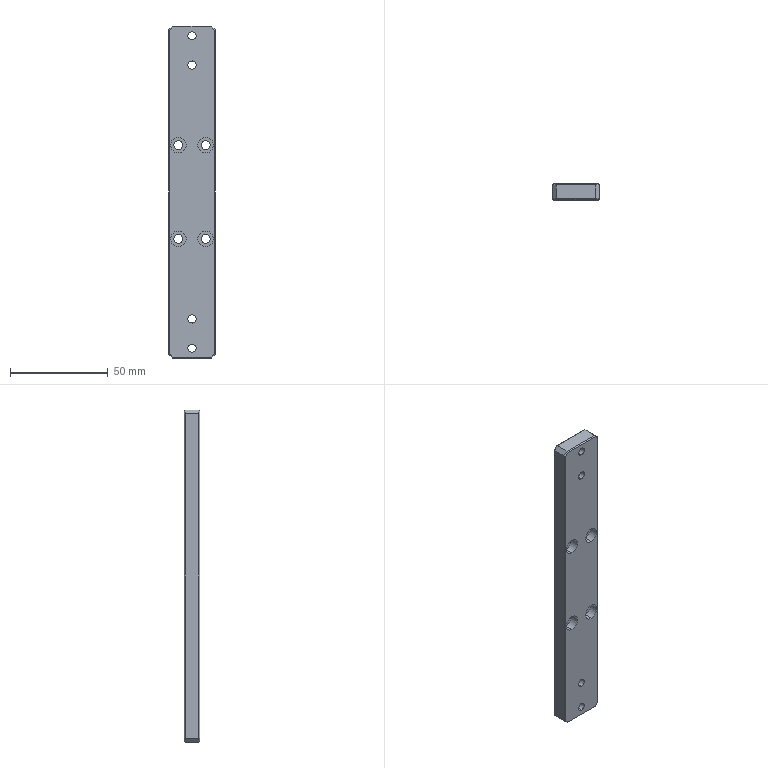Part | SolidWorks | features Chamfer 2, HoleWzd 2, Extrusion 1 | 1 solid | 54 faces | box 24 x 8 x 170 mm | volume 30923 mm3 | plane 30 | cylinder 24 | commonest cylinder face diameters 4.2 x8 4.5 x8 8 x8
STEP:
#1=CARTESIAN_POINT('',(0.,0.,-82.1));
#2=VERTEX_POINT('',#1);
#3=CARTESIAN_POINT('',(0.,0.,-77.9));
#4=VERTEX_POINT('',#3);
#5=CARTESIAN_POINT('',(0.,0.,-80.));
#6=DIRECTION('',(0.,1.,0.));
#7=DIRECTION('',(0.,0.,1.));
#8=AXIS2_PLACEMENT_3D('',#5,#6,#7);
#9=CIRCLE('',#8,2.1);
#10=EDGE_CURVE('',#2,#4,#9,.T.);
#11=ORIENTED_EDGE('',*,*,#10,.F.);
#12=CARTESIAN_POINT('',(0.,8.,-82.1));
#13=VERTEX_POINT('',#12);
#14=CARTESIAN_POINT('',(0.,8.,-82.1));
#15=DIRECTION('',(0.,1.,0.));
#16=VECTOR('',#15,1000.);
#17=LINE('',#14,#16);
#18=EDGE_CURVE('',#2,#13,#17,.T.);
#19=ORIENTED_EDGE('',*,*,#18,.T.);
#20=CARTESIAN_POINT('',(0.,8.,-77.9));
#21=VERTEX_POINT('',#20);
#22=CARTESIAN_POINT('',(0.,8.,-80.));
#23=DIRECTION('',(0.,1.,0.));
#24=DIRECTION('',(0.,0.,1.));
#25=AXIS2_PLACEMENT_3D('',#22,#23,#24);
#26=CIRCLE('',#25,2.1);
#27=EDGE_CURVE('',#13,#21,#26,.T.);
#28=ORIENTED_EDGE('',*,*,#27,.T.);
#29=CARTESIAN_POINT('',(0.,8.,-77.9));
#30=DIRECTION('',(0.,1.,0.));
#31=VECTOR('',#30,1000.);
#32=LINE('',#29,#31);
#33=EDGE_CURVE('',#4,#21,#32,.T.);
#34=ORIENTED_EDGE('',*,*,#33,.F.);
#35=EDGE_LOOP('',(#11,#19,#28,#34));
#36=FACE_OUTER_BOUND('',#35,.T.);
#37=CARTESIAN_POINT('',(0.,8.,-80.));
#38=DIRECTION('',(0.,1.,0.));
#39=DIRECTION('',(0.,0.,1.));
#40=AXIS2_PLACEMENT_3D('',#37,#38,#39);
#41=CYLINDRICAL_SURFACE('',#40,2.1);
#42=ADVANCED_FACE('',(#36),#41,.F.);
#43=CARTESIAN_POINT('',(0.,0.,77.9));
#44=VERTEX_POINT('',#43);
#45=CARTESIAN_POINT('',(0.,0.,82.1));
#46=VERTEX_POINT('',#45);
#47=CARTESIAN_POINT('',(0.,0.,80.));
#48=DIRECTION('',(0.,1.,0.));
#49=DIRECTION('',(0.,0.,1.));
#50=AXIS2_PLACEMENT_3D('',#47,#48,#49);
#51=CIRCLE('',#50,2.1);
#52=EDGE_CURVE('',#44,#46,#51,.T.);
#53=ORIENTED_EDGE('',*,*,#52,.F.);
#54=CARTESIAN_POINT('',(0.,8.,77.9));
#55=VERTEX_POINT('',#54);
#56=CARTESIAN_POINT('',(0.,8.,77.9));
#57=DIRECTION('',(0.,1.,0.));
#58=VECTOR('',#57,1000.);
#59=LINE('',#56,#58);
#60=EDGE_CURVE('',#44,#55,#59,.T.);
#61=ORIENTED_EDGE('',*,*,#60,.T.);
#62=CARTESIAN_POINT('',(0.,8.,82.1));
#63=VERTEX_POINT('',#62);
#64=CARTESIAN_POINT('',(0.,8.,80.));
#65=DIRECTION('',(0.,1.,0.));
#66=DIRECTION('',(0.,0.,1.));
#67=AXIS2_PLACEMENT_3D('',#64,#65,#66);
#68=CIRCLE('',#67,2.1);
#69=EDGE_CURVE('',#55,#63,#68,.T.);
#70=ORIENTED_EDGE('',*,*,#69,.T.);
#71=CARTESIAN_POINT('',(0.,8.,82.1));
#72=DIRECTION('',(0.,1.,0.));
#73=VECTOR('',#72,1000.);
#74=LINE('',#71,#73);
#75=EDGE_CURVE('',#46,#63,#74,.T.);
#76=ORIENTED_EDGE('',*,*,#75,.F.);
#77=EDGE_LOOP('',(#53,#61,#70,#76));
#78=FACE_OUTER_BOUND('',#77,.T.);
#79=CARTESIAN_POINT('',(0.,8.,80.));
#80=DIRECTION('',(0.,1.,0.));
#81=DIRECTION('',(0.,0.,1.));
#82=AXIS2_PLACEMENT_3D('',#79,#80,#81);
#83=CYLINDRICAL_SURFACE('',#82,2.1);
#84=ADVANCED_FACE('',(#78),#83,.F.);
#85=CARTESIAN_POINT('',(0.,0.,62.9));
#86=VERTEX_POINT('',#85);
#87=CARTESIAN_POINT('',(0.,0.,67.1));
#88=VERTEX_POINT('',#87);
#89=CARTESIAN_POINT('',(0.,0.,65.));
#90=DIRECTION('',(0.,1.,0.));
#91=DIRECTION('',(0.,0.,1.));
#92=AXIS2_PLACEMENT_3D('',#89,#90,#91);
#93=CIRCLE('',#92,2.1);
#94=EDGE_CURVE('',#86,#88,#93,.T.);
#95=ORIENTED_EDGE('',*,*,#94,.F.);
#96=CARTESIAN_POINT('',(0.,8.,62.9));
#97=VERTEX_POINT('',#96);
#98=CARTESIAN_POINT('',(0.,8.,62.9));
#99=DIRECTION('',(0.,1.,0.));
#100=VECTOR('',#99,1000.);
#101=LINE('',#98,#100);
#102=EDGE_CURVE('',#86,#97,#101,.T.);
#103=ORIENTED_EDGE('',*,*,#102,.T.);
#104=CARTESIAN_POINT('',(0.,8.,67.1));
#105=VERTEX_POINT('',#104);
#106=CARTESIAN_POINT('',(0.,8.,65.));
#107=DIRECTION('',(0.,1.,0.));
#108=DIRECTION('',(0.,0.,1.));
#109=AXIS2_PLACEMENT_3D('',#106,#107,#108);
#110=CIRCLE('',#109,2.1);
#111=EDGE_CURVE('',#97,#105,#110,.T.);
#112=ORIENTED_EDGE('',*,*,#111,.T.);
#113=CARTESIAN_POINT('',(0.,8.,67.1));
#114=DIRECTION('',(0.,1.,0.));
#115=VECTOR('',#114,1000.);
#116=LINE('',#113,#115);
#117=EDGE_CURVE('',#88,#105,#116,.T.);
#118=ORIENTED_EDGE('',*,*,#117,.F.);
#119=EDGE_LOOP('',(#95,#103,#112,#118));
#120=FACE_OUTER_BOUND('',#119,.T.);
#121=CARTESIAN_POINT('',(0.,8.,65.));
#122=DIRECTION('',(0.,1.,0.));
#123=DIRECTION('',(0.,0.,1.));
#124=AXIS2_PLACEMENT_3D('',#121,#122,#123);
#125=CYLINDRICAL_SURFACE('',#124,2.1);
#126=ADVANCED_FACE('',(#120),#125,.F.);
#127=CARTESIAN_POINT('',(0.,0.,-67.1));
#128=VERTEX_POINT('',#127);
#129=CARTESIAN_POINT('',(0.,0.,-62.9));
#130=VERTEX_POINT('',#129);
#131=CARTESIAN_POINT('',(0.,0.,-65.));
#132=DIRECTION('',(0.,1.,0.));
#133=DIRECTION('',(0.,0.,1.));
#134=AXIS2_PLACEMENT_3D('',#131,#132,#133);
#135=CIRCLE('',#134,2.1);
#136=EDGE_CURVE('',#128,#130,#135,.T.);
#137=ORIENTED_EDGE('',*,*,#136,.F.);
#138=CARTESIAN_POINT('',(0.,8.,-67.1));
#139=VERTEX_POINT('',#138);
#140=CARTESIAN_POINT('',(0.,8.,-67.1));
#141=DIRECTION('',(0.,1.,0.));
#142=VECTOR('',#141,1000.);
#143=LINE('',#140,#142);
#144=EDGE_CURVE('',#128,#139,#143,.T.);
#145=ORIENTED_EDGE('',*,*,#144,.T.);
#146=CARTESIAN_POINT('',(0.,8.,-62.9));
#147=VERTEX_POINT('',#146);
#148=CARTESIAN_POINT('',(0.,8.,-65.));
#149=DIRECTION('',(0.,1.,0.));
#150=DIRECTION('',(0.,0.,1.));
#151=AXIS2_PLACEMENT_3D('',#148,#149,#150);
#152=CIRCLE('',#151,2.1);
#153=EDGE_CURVE('',#139,#147,#152,.T.);
#154=ORIENTED_EDGE('',*,*,#153,.T.);
#155=CARTESIAN_POINT('',(0.,8.,-62.9));
#156=DIRECTION('',(0.,1.,0.));
#157=VECTOR('',#156,1000.);
#158=LINE('',#155,#157);
#159=EDGE_CURVE('',#130,#147,#158,.T.);
#160=ORIENTED_EDGE('',*,*,#159,.F.);
#161=EDGE_LOOP('',(#137,#145,#154,#160));
#162=FACE_OUTER_BOUND('',#161,.T.);
#163=CARTESIAN_POINT('',(0.,8.,-65.));
#164=DIRECTION('',(0.,1.,0.));
#165=DIRECTION('',(0.,0.,1.));
#166=AXIS2_PLACEMENT_3D('',#163,#164,#165);
#167=CYLINDRICAL_SURFACE('',#166,2.1);
#168=ADVANCED_FACE('',(#162),#167,.F.);
#169=CARTESIAN_POINT('',(7.,4.4,-20.));
#170=VERTEX_POINT('',#169);
#171=CARTESIAN_POINT('',(7.,4.4,-28.));
#172=VERTEX_POINT('',#171);
#173=CARTESIAN_POINT('',(7.,4.4,-24.));
#174=DIRECTION('',(0.,-1.,0.));
#175=DIRECTION('',(0.,0.,-1.));
#176=AXIS2_PLACEMENT_3D('',#173,#174,#175);
#177=CIRCLE('',#176,4.);
#178=EDGE_CURVE('',#170,#172,#177,.T.);
#179=ORIENTED_EDGE('',*,*,#178,.F.);
#180=CARTESIAN_POINT('',(7.,0.,-20.));
#181=VERTEX_POINT('',#180);
#182=CARTESIAN_POINT('',(7.,0.,-20.));
#183=DIRECTION('',(0.,-1.,0.));
#184=VECTOR('',#183,1000.);
#185=LINE('',#182,#184);
#186=EDGE_CURVE('',#170,#181,#185,.T.);
#187=ORIENTED_EDGE('',*,*,#186,.T.);
#188=CARTESIAN_POINT('',(7.,0.,-28.));
#189=VERTEX_POINT('',#188);
#190=CARTESIAN_POINT('',(7.,0.,-24.));
#191=DIRECTION('',(0.,-1.,0.));
#192=DIRECTION('',(0.,0.,-1.));
#193=AXIS2_PLACEMENT_3D('',#190,#191,#192);
#194=CIRCLE('',#193,4.);
#195=EDGE_CURVE('',#181,#189,#194,.T.);
#196=ORIENTED_EDGE('',*,*,#195,.T.);
#197=CARTESIAN_POINT('',(7.,0.,-28.));
#198=DIRECTION('',(0.,-1.,0.));
#199=VECTOR('',#198,1000.);
#200=LINE('',#197,#199);
#201=EDGE_CURVE('',#172,#189,#200,.T.);
#202=ORIENTED_EDGE('',*,*,#201,.F.);
#203=EDGE_LOOP('',(#179,#187,#196,#202));
#204=FACE_OUTER_BOUND('',#203,.T.);
#205=CARTESIAN_POINT('',(7.,0.,-24.));
#206=DIRECTION('',(0.,-1.,0.));
#207=DIRECTION('',(0.,0.,-1.));
#208=AXIS2_PLACEMENT_3D('',#205,#206,#207);
#209=CYLINDRICAL_SURFACE('',#208,4.);
#210=ADVANCED_FACE('',(#204),#209,.F.);
#211=CARTESIAN_POINT('',(7.,8.,-21.75));
#212=VERTEX_POINT('',#211);
#213=CARTESIAN_POINT('',(7.,8.,-26.25));
#214=VERTEX_POINT('',#213);
#215=CARTESIAN_POINT('',(7.,8.,-24.));
#216=DIRECTION('',(0.,-1.,0.));
#217=DIRECTION('',(0.,0.,-1.));
#218=AXIS2_PLACEMENT_3D('',#215,#216,#217);
#219=CIRCLE('',#218,2.25);
#220=EDGE_CURVE('',#212,#214,#219,.T.);
#221=ORIENTED_EDGE('',*,*,#220,.F.);
#222=CARTESIAN_POINT('',(7.,4.4,-21.75));
#223=VERTEX_POINT('',#222);
#224=CARTESIAN_POINT('',(7.,0.,-21.75));
#225=DIRECTION('',(0.,-1.,0.));
#226=VECTOR('',#225,1000.);
#227=LINE('',#224,#226);
#228=EDGE_CURVE('',#212,#223,#227,.T.);
#229=ORIENTED_EDGE('',*,*,#228,.T.);
#230=CARTESIAN_POINT('',(7.,4.4,-26.25));
#231=VERTEX_POINT('',#230);
#232=CARTESIAN_POINT('',(7.,4.4,-24.));
#233=DIRECTION('',(0.,-1.,0.));
#234=DIRECTION('',(0.,0.,-1.));
#235=AXIS2_PLACEMENT_3D('',#232,#233,#234);
#236=CIRCLE('',#235,2.25);
#237=EDGE_CURVE('',#223,#231,#236,.T.);
#238=ORIENTED_EDGE('',*,*,#237,.T.);
#239=CARTESIAN_POINT('',(7.,0.,-26.25));
#240=DIRECTION('',(0.,-1.,0.));
#241=VECTOR('',#240,1000.);
#242=LINE('',#239,#241);
#243=EDGE_CURVE('',#214,#231,#242,.T.);
#244=ORIENTED_EDGE('',*,*,#243,.F.);
#245=EDGE_LOOP('',(#221,#229,#238,#244));
#246=FACE_OUTER_BOUND('',#245,.T.);
#247=CARTESIAN_POINT('',(7.,0.,-24.));
#248=DIRECTION('',(0.,-1.,0.));
#249=DIRECTION('',(0.,0.,-1.));
#250=AXIS2_PLACEMENT_3D('',#247,#248,#249);
#251=CYLINDRICAL_SURFACE('',#250,2.25);
#252=ADVANCED_FACE('',(#246),#251,.F.);
#253=CARTESIAN_POINT('',(-7.,4.4,-20.));
#254=VERTEX_POINT('',#253);
#255=CARTESIAN_POINT('',(-7.,4.4,-28.));
#256=VERTEX_POINT('',#255);
#257=CARTESIAN_POINT('',(-7.,4.4,-24.));
#258=DIRECTION('',(0.,-1.,0.));
#259=DIRECTION('',(0.,0.,-1.));
#260=AXIS2_PLACEMENT_3D('',#257,#258,#259);
#261=CIRCLE('',#260,4.);
#262=EDGE_CURVE('',#254,#256,#261,.T.);
#263=ORIENTED_EDGE('',*,*,#262,.F.);
#264=CARTESIAN_POINT('',(-7.,0.,-20.));
#265=VERTEX_POINT('',#264);
#266=CARTESIAN_POINT('',(-7.,0.,-20.));
#267=DIRECTION('',(0.,-1.,0.));
#268=VECTOR('',#267,1000.);
#269=LINE('',#266,#268);
#270=EDGE_CURVE('',#254,#265,#269,.T.);
#271=ORIENTED_EDGE('',*,*,#270,.T.);
#272=CARTESIAN_POINT('',(-7.,0.,-28.));
#273=VERTEX_POINT('',#272);
#274=CARTESIAN_POINT('',(-7.,0.,-24.));
#275=DIRECTION('',(0.,-1.,0.));
#276=DIRECTION('',(0.,0.,-1.));
#277=AXIS2_PLACEMENT_3D('',#274,#275,#276);
#278=CIRCLE('',#277,4.);
#279=EDGE_CURVE('',#265,#273,#278,.T.);
#280=ORIENTED_EDGE('',*,*,#279,.T.);
#281=CARTESIAN_POINT('',(-7.,0.,-28.));
#282=DIRECTION('',(0.,-1.,0.));
#283=VECTOR('',#282,1000.);
#284=LINE('',#281,#283);
#285=EDGE_CURVE('',#256,#273,#284,.T.);
#286=ORIENTED_EDGE('',*,*,#285,.F.);
#287=EDGE_LOOP('',(#263,#271,#280,#286));
#288=FACE_OUTER_BOUND('',#287,.T.);
#289=CARTESIAN_POINT('',(-7.,0.,-24.));
#290=DIRECTION('',(0.,-1.,0.));
#291=DIRECTION('',(0.,0.,-1.));
#292=AXIS2_PLACEMENT_3D('',#289,#290,#291);
#293=CYLINDRICAL_SURFACE('',#292,4.);
#294=ADVANCED_FACE('',(#288),#293,.F.);
#295=CARTESIAN_POINT('',(-7.,8.,-21.75));
#296=VERTEX_POINT('',#295);
#297=CARTESIAN_POINT('',(-7.,8.,-26.25));
#298=VERTEX_POINT('',#297);
#299=CARTESIAN_POINT('',(-7.,8.,-24.));
#300=DIRECTION('',(0.,-1.,0.));
#301=DIRECTION('',(0.,0.,-1.));
#302=AXIS2_PLACEMENT_3D('',#299,#300,#301);
#303=CIRCLE('',#302,2.25);
#304=EDGE_CURVE('',#296,#298,#303,.T.);
#305=ORIENTED_EDGE('',*,*,#304,.F.);
#306=CARTESIAN_POINT('',(-7.,4.4,-21.75));
#307=VERTEX_POINT('',#306);
#308=CARTESIAN_POINT('',(-7.,0.,-21.75));
#309=DIRECTION('',(0.,-1.,0.));
#310=VECTOR('',#309,1000.);
#311=LINE('',#308,#310);
#312=EDGE_CURVE('',#296,#307,#311,.T.);
#313=ORIENTED_EDGE('',*,*,#312,.T.);
#314=CARTESIAN_POINT('',(-7.,4.4,-26.25));
#315=VERTEX_POINT('',#314);
#316=CARTESIAN_POINT('',(-7.,4.4,-24.));
#317=DIRECTION('',(0.,-1.,0.));
#318=DIRECTION('',(0.,0.,-1.));
#319=AXIS2_PLACEMENT_3D('',#316,#317,#318);
#320=CIRCLE('',#319,2.25);
#321=EDGE_CURVE('',#307,#315,#320,.T.);
#322=ORIENTED_EDGE('',*,*,#321,.T.);
#323=CARTESIAN_POINT('',(-7.,0.,-26.25));
#324=DIRECTION('',(0.,-1.,0.));
#325=VECTOR('',#324,1000.);
#326=LINE('',#323,#325);
#327=EDGE_CURVE('',#298,#315,#326,.T.);
#328=ORIENTED_EDGE('',*,*,#327,.F.);
#329=EDGE_LOOP('',(#305,#313,#322,#328));
#330=FACE_OUTER_BOUND('',#329,.T.);
#331=CARTESIAN_POINT('',(-7.,0.,-24.));
#332=DIRECTION('',(0.,-1.,0.));
#333=DIRECTION('',(0.,0.,-1.));
#334=AXIS2_PLACEMENT_3D('',#331,#332,#333);
#335=CYLINDRICAL_SURFACE('',#334,2.25);
#336=ADVANCED_FACE('',(#330),#335,.F.);
#337=CARTESIAN_POINT('',(7.,4.4,28.));
#338=VERTEX_POINT('',#337);
#339=CARTESIAN_POINT('',(7.,4.4,20.));
#340=VERTEX_POINT('',#339);
#341=CARTESIAN_POINT('',(7.,4.4,24.));
#342=DIRECTION('',(0.,-1.,0.));
#343=DIRECTION('',(0.,0.,-1.));
#344=AXIS2_PLACEMENT_3D('',#341,#342,#343);
#345=CIRCLE('',#344,4.);
#346=EDGE_CURVE('',#338,#340,#345,.T.);
#347=ORIENTED_EDGE('',*,*,#346,.F.);
#348=CARTESIAN_POINT('',(7.,0.,28.));
#349=VERTEX_POINT('',#348);
#350=CARTESIAN_POINT('',(7.,0.,28.));
#351=DIRECTION('',(0.,-1.,0.));
#352=VECTOR('',#351,1000.);
#353=LINE('',#350,#352);
#354=EDGE_CURVE('',#338,#349,#353,.T.);
#355=ORIENTED_EDGE('',*,*,#354,.T.);
#356=CARTESIAN_POINT('',(7.,0.,20.));
#357=VERTEX_POINT('',#356);
#358=CARTESIAN_POINT('',(7.,0.,24.));
#359=DIRECTION('',(0.,-1.,0.));
#360=DIRECTION('',(0.,0.,-1.));
#361=AXIS2_PLACEMENT_3D('',#358,#359,#360);
#362=CIRCLE('',#361,4.);
#363=EDGE_CURVE('',#349,#357,#362,.T.);
#364=ORIENTED_EDGE('',*,*,#363,.T.);
#365=CARTESIAN_POINT('',(7.,0.,20.));
#366=DIRECTION('',(0.,-1.,0.));
#367=VECTOR('',#366,1000.);
#368=LINE('',#365,#367);
#369=EDGE_CURVE('',#340,#357,#368,.T.);
#370=ORIENTED_EDGE('',*,*,#369,.F.);
#371=EDGE_LOOP('',(#347,#355,#364,#370));
#372=FACE_OUTER_BOUND('',#371,.T.);
#373=CARTESIAN_POINT('',(7.,0.,24.));
#374=DIRECTION('',(0.,-1.,0.));
#375=DIRECTION('',(0.,0.,-1.));
#376=AXIS2_PLACEMENT_3D('',#373,#374,#375);
#377=CYLINDRICAL_SURFACE('',#376,4.);
#378=ADVANCED_FACE('',(#372),#377,.F.);
#379=CARTESIAN_POINT('',(7.,8.,26.25));
#380=VERTEX_POINT('',#379);
#381=CARTESIAN_POINT('',(7.,8.,21.75));
#382=VERTEX_POINT('',#381);
#383=CARTESIAN_POINT('',(7.,8.,24.));
#384=DIRECTION('',(0.,-1.,0.));
#385=DIRECTION('',(0.,0.,-1.));
#386=AXIS2_PLACEMENT_3D('',#383,#384,#385);
#387=CIRCLE('',#386,2.25);
#388=EDGE_CURVE('',#380,#382,#387,.T.);
#389=ORIENTED_EDGE('',*,*,#388,.F.);
#390=CARTESIAN_POINT('',(7.,4.4,26.25));
#391=VERTEX_POINT('',#390);
#392=CARTESIAN_POINT('',(7.,0.,26.25));
#393=DIRECTION('',(0.,-1.,0.));
#394=VECTOR('',#393,1000.);
#395=LINE('',#392,#394);
#396=EDGE_CURVE('',#380,#391,#395,.T.);
#397=ORIENTED_EDGE('',*,*,#396,.T.);
#398=CARTESIAN_POINT('',(7.,4.4,21.75));
#399=VERTEX_POINT('',#398);
#400=CARTESIAN_POINT('',(7.,4.4,24.));
#401=DIRECTION('',(0.,-1.,0.));
#402=DIRECTION('',(0.,0.,-1.));
#403=AXIS2_PLACEMENT_3D('',#400,#401,#402);
#404=CIRCLE('',#403,2.25);
#405=EDGE_CURVE('',#391,#399,#404,.T.);
#406=ORIENTED_EDGE('',*,*,#405,.T.);
#407=CARTESIAN_POINT('',(7.,0.,21.75));
#408=DIRECTION('',(0.,-1.,0.));
#409=VECTOR('',#408,1000.);
#410=LINE('',#407,#409);
#411=EDGE_CURVE('',#382,#399,#410,.T.);
#412=ORIENTED_EDGE('',*,*,#411,.F.);
#413=EDGE_LOOP('',(#389,#397,#406,#412));
#414=FACE_OUTER_BOUND('',#413,.T.);
#415=CARTESIAN_POINT('',(7.,0.,24.));
#416=DIRECTION('',(0.,-1.,0.));
#417=DIRECTION('',(0.,0.,-1.));
#418=AXIS2_PLACEMENT_3D('',#415,#416,#417);
#419=CYLINDRICAL_SURFACE('',#418,2.25);
#420=ADVANCED_FACE('',(#414),#419,.F.);
#421=CARTESIAN_POINT('',(-7.,4.4,28.));
#422=VERTEX_POINT('',#421);
#423=CARTESIAN_POINT('',(-7.,4.4,20.));
#424=VERTEX_POINT('',#423);
#425=CARTESIAN_POINT('',(-7.,4.4,24.));
#426=DIRECTION('',(0.,-1.,0.));
#427=DIRECTION('',(0.,0.,-1.));
#428=AXIS2_PLACEMENT_3D('',#425,#426,#427);
#429=CIRCLE('',#428,4.);
#430=EDGE_CURVE('',#422,#424,#429,.T.);
#431=ORIENTED_EDGE('',*,*,#430,.F.);
#432=CARTESIAN_POINT('',(-7.,0.,28.));
#433=VERTEX_POINT('',#432);
#434=CARTESIAN_POINT('',(-7.,0.,28.));
#435=DIRECTION('',(0.,-1.,0.));
#436=VECTOR('',#435,1000.);
#437=LINE('',#434,#436);
#438=EDGE_CURVE('',#422,#433,#437,.T.);
#439=ORIENTED_EDGE('',*,*,#438,.T.);
#440=CARTESIAN_POINT('',(-7.,0.,20.));
#441=VERTEX_POINT('',#440);
#442=CARTESIAN_POINT('',(-7.,0.,24.));
#443=DIRECTION('',(0.,-1.,0.));
#444=DIRECTION('',(0.,0.,-1.));
#445=AXIS2_PLACEMENT_3D('',#442,#443,#444);
#446=CIRCLE('',#445,4.);
#447=EDGE_CURVE('',#433,#441,#446,.T.);
#448=ORIENTED_EDGE('',*,*,#447,.T.);
#449=CARTESIAN_POINT('',(-7.,0.,20.));
#450=DIRECTION('',(0.,-1.,0.));
#451=VECTOR('',#450,1000.);
#452=LINE('',#449,#451);
#453=EDGE_CURVE('',#424,#441,#452,.T.);
#454=ORIENTED_EDGE('',*,*,#453,.F.);
#455=EDGE_LOOP('',(#431,#439,#448,#454));
#456=FACE_OUTER_BOUND('',#455,.T.);
#457=CARTESIAN_POINT('',(-7.,0.,24.));
#458=DIRECTION('',(0.,-1.,0.));
#459=DIRECTION('',(0.,0.,-1.));
#460=AXIS2_PLACEMENT_3D('',#457,#458,#459);
#461=CYLINDRICAL_SURFACE('',#460,4.);
#462=ADVANCED_FACE('',(#456),#461,.F.);
#463=CARTESIAN_POINT('',(-7.,8.,26.25));
#464=VERTEX_POINT('',#463);
#465=CARTESIAN_POINT('',(-7.,8.,21.75));
#466=VERTEX_POINT('',#465);
#467=CARTESIAN_POINT('',(-7.,8.,24.));
#468=DIRECTION('',(0.,-1.,0.));
#469=DIRECTION('',(0.,0.,-1.));
#470=AXIS2_PLACEMENT_3D('',#467,#468,#469);
#471=CIRCLE('',#470,2.25);
#472=EDGE_CURVE('',#464,#466,#471,.T.);
#473=ORIENTED_EDGE('',*,*,#472,.F.);
#474=CARTESIAN_POINT('',(-7.,4.4,26.25));
#475=VERTEX_POINT('',#474);
#476=CARTESIAN_POINT('',(-7.,0.,26.25));
#477=DIRECTION('',(0.,-1.,0.));
#478=VECTOR('',#477,1000.);
#479=LINE('',#476,#478);
#480=EDGE_CURVE('',#464,#475,#479,.T.);
#481=ORIENTED_EDGE('',*,*,#480,.T.);
#482=CARTESIAN_POINT('',(-7.,4.4,21.75));
#483=VERTEX_POINT('',#482);
#484=CARTESIAN_POINT('',(-7.,4.4,24.));
#485=DIRECTION('',(0.,-1.,0.));
#486=DIRECTION('',(0.,0.,-1.));
#487=AXIS2_PLACEMENT_3D('',#484,#485,#486);
#488=CIRCLE('',#487,2.25);
#489=EDGE_CURVE('',#475,#483,#488,.T.);
#490=ORIENTED_EDGE('',*,*,#489,.T.);
#491=CARTESIAN_POINT('',(-7.,0.,21.75));
#492=DIRECTION('',(0.,-1.,0.));
#493=VECTOR('',#492,1000.);
#494=LINE('',#491,#493);
#495=EDGE_CURVE('',#466,#483,#494,.T.);
#496=ORIENTED_EDGE('',*,*,#495,.F.);
#497=EDGE_LOOP('',(#473,#481,#490,#496));
#498=FACE_OUTER_BOUND('',#497,.T.);
#499=CARTESIAN_POINT('',(-7.,0.,24.));
#500=DIRECTION('',(0.,-1.,0.));
#501=DIRECTION('',(0.,0.,-1.));
#502=AXIS2_PLACEMENT_3D('',#499,#500,#501);
#503=CYLINDRICAL_SURFACE('',#502,2.25);
#504=ADVANCED_FACE('',(#498),#503,.F.);
#505=CARTESIAN_POINT('',(12.,7.5,83.));
#506=VERTEX_POINT('',#505);
#507=CARTESIAN_POINT('',(12.,0.5,83.));
#508=VERTEX_POINT('',#507);
#509=CARTESIAN_POINT('',(12.,8.,83.));
#510=DIRECTION('',(0.,-1.,0.));
#511=VECTOR('',#510,1000.);
#512=LINE('',#509,#511);
#513=EDGE_CURVE('',#506,#508,#512,.T.);
#514=ORIENTED_EDGE('',*,*,#513,.T.);
#515=CARTESIAN_POINT('',(12.,0.5,-83.));
#516=VERTEX_POINT('',#515);
#517=CARTESIAN_POINT('',(12.,0.5,-85.));
#518=DIRECTION('',(0.,0.,-1.));
#519=VECTOR('',#518,1000.);
#520=LINE('',#517,#519);
#521=EDGE_CURVE('',#508,#516,#520,.T.);
#522=ORIENTED_EDGE('',*,*,#521,.T.);
#523=CARTESIAN_POINT('',(12.,7.5,-83.));
#524=VERTEX_POINT('',#523);
#525=CARTESIAN_POINT('',(12.,8.,-83.));
#526=DIRECTION('',(0.,1.,0.));
#527=VECTOR('',#526,1000.);
#528=LINE('',#525,#527);
#529=EDGE_CURVE('',#516,#524,#528,.T.);
#530=ORIENTED_EDGE('',*,*,#529,.T.);
#531=CARTESIAN_POINT('',(12.,7.5,83.));
#532=DIRECTION('',(0.,0.,1.));
#533=VECTOR('',#532,1000.);
#534=LINE('',#531,#533);
#535=EDGE_CURVE('',#524,#506,#534,.T.);
#536=ORIENTED_EDGE('',*,*,#535,.T.);
#537=EDGE_LOOP('',(#514,#522,#530,#536));
#538=FACE_OUTER_BOUND('',#537,.T.);
#539=CARTESIAN_POINT('',(12.,8.,-85.));
#540=DIRECTION('',(-1.,0.,0.));
#541=DIRECTION('',(0.,0.,1.));
#542=AXIS2_PLACEMENT_3D('',#539,#540,#541);
#543=PLANE('',#542);
#544=ADVANCED_FACE('',(#538),#543,.F.);
#545=CARTESIAN_POINT('',(10.,7.5,-85.));
#546=VERTEX_POINT('',#545);
#547=CARTESIAN_POINT('',(10.,0.5,-85.));
#548=VERTEX_POINT('',#547);
#549=CARTESIAN_POINT('',(10.,8.,-85.));
#550=DIRECTION('',(0.,-1.,0.));
#551=VECTOR('',#550,1000.);
#552=LINE('',#549,#551);
#553=EDGE_CURVE('',#546,#548,#552,.T.);
#554=ORIENTED_EDGE('',*,*,#553,.T.);
#555=CARTESIAN_POINT('',(-10.,0.5,-85.));
#556=VERTEX_POINT('',#555);
#557=CARTESIAN_POINT('',(-12.,0.5,-85.));
#558=DIRECTION('',(-1.,0.,0.));
#559=VECTOR('',#558,1000.);
#560=LINE('',#557,#559);
#561=EDGE_CURVE('',#548,#556,#560,.T.);
#562=ORIENTED_EDGE('',*,*,#561,.T.);
#563=CARTESIAN_POINT('',(-10.,7.5,-85.));
#564=VERTEX_POINT('',#563);
#565=CARTESIAN_POINT('',(-10.,8.,-85.));
#566=DIRECTION('',(0.,1.,0.));
#567=VECTOR('',#566,1000.);
#568=LINE('',#565,#567);
#569=EDGE_CURVE('',#556,#564,#568,.T.);
#570=ORIENTED_EDGE('',*,*,#569,.T.);
#571=CARTESIAN_POINT('',(10.,7.5,-85.));
#572=DIRECTION('',(1.,0.,0.));
#573=VECTOR('',#572,1000.);
#574=LINE('',#571,#573);
#575=EDGE_CURVE('',#564,#546,#574,.T.);
#576=ORIENTED_EDGE('',*,*,#575,.T.);
#577=EDGE_LOOP('',(#554,#562,#570,#576));
#578=FACE_OUTER_BOUND('',#577,.T.);
#579=CARTESIAN_POINT('',(-12.,8.,-85.));
#580=DIRECTION('',(0.,0.,1.));
#581=DIRECTION('',(1.,0.,0.));
#582=AXIS2_PLACEMENT_3D('',#579,#580,#581);
#583=PLANE('',#582);
#584=ADVANCED_FACE('',(#578),#583,.F.);
#585=CARTESIAN_POINT('',(-12.,7.5,-83.));
#586=VERTEX_POINT('',#585);
#587=CARTESIAN_POINT('',(-12.,0.5,-83.));
#588=VERTEX_POINT('',#587);
#589=CARTESIAN_POINT('',(-12.,8.,-83.));
#590=DIRECTION('',(0.,-1.,0.));
#591=VECTOR('',#590,1000.);
#592=LINE('',#589,#591);
#593=EDGE_CURVE('',#586,#588,#592,.T.);
#594=ORIENTED_EDGE('',*,*,#593,.T.);
#595=CARTESIAN_POINT('',(-12.,0.5,83.));
#596=VERTEX_POINT('',#595);
#597=CARTESIAN_POINT('',(-12.,0.5,-85.));
#598=DIRECTION('',(0.,0.,1.));
#599=VECTOR('',#598,1000.);
#600=LINE('',#597,#599);
#601=EDGE_CURVE('',#588,#596,#600,.T.);
#602=ORIENTED_EDGE('',*,*,#601,.T.);
#603=CARTESIAN_POINT('',(-12.,7.5,83.));
#604=VERTEX_POINT('',#603);
#605=CARTESIAN_POINT('',(-12.,8.,83.));
#606=DIRECTION('',(0.,1.,0.));
#607=VECTOR('',#606,1000.);
#608=LINE('',#605,#607);
#609=EDGE_CURVE('',#596,#604,#608,.T.);
#610=ORIENTED_EDGE('',*,*,#609,.T.);
#611=CARTESIAN_POINT('',(-12.,7.5,-83.));
#612=DIRECTION('',(0.,0.,-1.));
#613=VECTOR('',#612,1000.);
#614=LINE('',#611,#613);
#615=EDGE_CURVE('',#604,#586,#614,.T.);
#616=ORIENTED_EDGE('',*,*,#615,.T.);
#617=EDGE_LOOP('',(#594,#602,#610,#616));
#618=FACE_OUTER_BOUND('',#617,.T.);
#619=CARTESIAN_POINT('',(-12.,8.,-85.));
#620=DIRECTION('',(1.,0.,0.));
#621=DIRECTION('',(0.,0.,-1.));
#622=AXIS2_PLACEMENT_3D('',#619,#620,#621);
#623=PLANE('',#622);
#624=ADVANCED_FACE('',(#618),#623,.F.);
#625=CARTESIAN_POINT('',(-10.,7.5,85.));
#626=VERTEX_POINT('',#625);
#627=CARTESIAN_POINT('',(-10.,0.5,85.));
#628=VERTEX_POINT('',#627);
#629=CARTESIAN_POINT('',(-10.,8.,85.));
#630=DIRECTION('',(0.,-1.,0.));
#631=VECTOR('',#630,1000.);
#632=LINE('',#629,#631);
#633=EDGE_CURVE('',#626,#628,#632,.T.);
#634=ORIENTED_EDGE('',*,*,#633,.T.);
#635=CARTESIAN_POINT('',(10.,0.5,85.));
#636=VERTEX_POINT('',#635);
#637=CARTESIAN_POINT('',(-12.,0.5,85.));
#638=DIRECTION('',(1.,0.,0.));
#639=VECTOR('',#638,1000.);
#640=LINE('',#637,#639);
#641=EDGE_CURVE('',#628,#636,#640,.T.);
#642=ORIENTED_EDGE('',*,*,#641,.T.);
#643=CARTESIAN_POINT('',(10.,7.5,85.));
#644=VERTEX_POINT('',#643);
#645=CARTESIAN_POINT('',(10.,8.,85.));
#646=DIRECTION('',(0.,1.,0.));
#647=VECTOR('',#646,1000.);
#648=LINE('',#645,#647);
#649=EDGE_CURVE('',#636,#644,#648,.T.);
#650=ORIENTED_EDGE('',*,*,#649,.T.);
#651=CARTESIAN_POINT('',(-10.,7.5,85.));
#652=DIRECTION('',(-1.,0.,0.));
#653=VECTOR('',#652,1000.);
#654=LINE('',#651,#653);
#655=EDGE_CURVE('',#644,#626,#654,.T.);
#656=ORIENTED_EDGE('',*,*,#655,.T.);
#657=EDGE_LOOP('',(#634,#642,#650,#656));
#658=FACE_OUTER_BOUND('',#657,.T.);
#659=CARTESIAN_POINT('',(-12.,8.,85.));
#660=DIRECTION('',(0.,0.,-1.));
#661=DIRECTION('',(-1.,0.,0.));
#662=AXIS2_PLACEMENT_3D('',#659,#660,#661);
#663=PLANE('',#662);
#664=ADVANCED_FACE('',(#658),#663,.F.);
#665=CARTESIAN_POINT('',(-9.793,8.,84.5));
#666=VERTEX_POINT('',#665);
#667=CARTESIAN_POINT('',(9.793,8.,84.5));
#668=VERTEX_POINT('',#667);
#669=CARTESIAN_POINT('',(10.,8.,84.5));
#670=DIRECTION('',(1.,0.,0.));
#671=VECTOR('',#670,1000.);
#672=LINE('',#669,#671);
#673=EDGE_CURVE('',#666,#668,#672,.T.);
#674=ORIENTED_EDGE('',*,*,#673,.T.);
#675=CARTESIAN_POINT('',(11.5,8.,82.793));
#676=VERTEX_POINT('',#675);
#677=CARTESIAN_POINT('',(47.146,8.,47.146));
#678=DIRECTION('',(0.7071,0.,-0.7071));
#679=VECTOR('',#678,1000.);
#680=LINE('',#677,#679);
#681=EDGE_CURVE('',#668,#676,#680,.T.);
#682=ORIENTED_EDGE('',*,*,#681,.T.);
#683=CARTESIAN_POINT('',(11.5,8.,-82.793));
#684=VERTEX_POINT('',#683);
#685=CARTESIAN_POINT('',(11.5,8.,-83.));
#686=DIRECTION('',(0.,0.,-1.));
#687=VECTOR('',#686,1000.);
#688=LINE('',#685,#687);
#689=EDGE_CURVE('',#676,#684,#688,.T.);
#690=ORIENTED_EDGE('',*,*,#689,.T.);
#691=CARTESIAN_POINT('',(9.793,8.,-84.5));
#692=VERTEX_POINT('',#691);
#693=CARTESIAN_POINT('',(47.146,8.,-47.146));
#694=DIRECTION('',(-0.7071,0.,-0.7071));
#695=VECTOR('',#694,1000.);
#696=LINE('',#693,#695);
#697=EDGE_CURVE('',#684,#692,#696,.T.);
#698=ORIENTED_EDGE('',*,*,#697,.T.);
#699=CARTESIAN_POINT('',(-9.793,8.,-84.5));
#700=VERTEX_POINT('',#699);
#701=CARTESIAN_POINT('',(-10.,8.,-84.5));
#702=DIRECTION('',(-1.,0.,0.));
#703=VECTOR('',#702,1000.);
#704=LINE('',#701,#703);
#705=EDGE_CURVE('',#692,#700,#704,.T.);
#706=ORIENTED_EDGE('',*,*,#705,.T.);
#707=CARTESIAN_POINT('',(-11.5,8.,-82.793));
#708=VERTEX_POINT('',#707);
#709=CARTESIAN_POINT('',(-47.146,8.,-47.146));
#710=DIRECTION('',(-0.7071,0.,0.7071));
#711=VECTOR('',#710,1000.);
#712=LINE('',#709,#711);
#713=EDGE_CURVE('',#700,#708,#712,.T.);
#714=ORIENTED_EDGE('',*,*,#713,.T.);
#715=CARTESIAN_POINT('',(-11.5,8.,82.793));
#716=VERTEX_POINT('',#715);
#717=CARTESIAN_POINT('',(-11.5,8.,83.));
#718=DIRECTION('',(0.,0.,1.));
#719=VECTOR('',#718,1000.);
#720=LINE('',#717,#719);
#721=EDGE_CURVE('',#708,#716,#720,.T.);
#722=ORIENTED_EDGE('',*,*,#721,.T.);
#723=CARTESIAN_POINT('',(-47.146,8.,47.146));
#724=DIRECTION('',(0.7071,0.,0.7071));
#725=VECTOR('',#724,1000.);
#726=LINE('',#723,#725);
#727=EDGE_CURVE('',#716,#666,#726,.T.);
#728=ORIENTED_EDGE('',*,*,#727,.T.);
#729=EDGE_LOOP('',(#674,#682,#690,#698,#706,#714,#722,#728));
#730=FACE_OUTER_BOUND('',#729,.T.);
#731=CARTESIAN_POINT('',(0.,8.,-80.));
#732=DIRECTION('',(0.,1.,0.));
#733=DIRECTION('',(0.,0.,1.));
#734=AXIS2_PLACEMENT_3D('',#731,#732,#733);
#735=CIRCLE('',#734,2.1);
#736=EDGE_CURVE('',#21,#13,#735,.T.);
#737=ORIENTED_EDGE('',*,*,#736,.F.);
#738=ORIENTED_EDGE('',*,*,#27,.F.);
#739=EDGE_LOOP('',(#737,#738));
#740=FACE_BOUND('',#739,.T.);
#741=CARTESIAN_POINT('',(0.,8.,80.));
#742=DIRECTION('',(0.,1.,0.));
#743=DIRECTION('',(0.,0.,1.));
#744=AXIS2_PLACEMENT_3D('',#741,#742,#743);
#745=CIRCLE('',#744,2.1);
#746=EDGE_CURVE('',#63,#55,#745,.T.);
#747=ORIENTED_EDGE('',*,*,#746,.F.);
#748=ORIENTED_EDGE('',*,*,#69,.F.);
#749=EDGE_LOOP('',(#747,#748));
#750=FACE_BOUND('',#749,.T.);
#751=CARTESIAN_POINT('',(0.,8.,65.));
#752=DIRECTION('',(0.,1.,0.));
#753=DIRECTION('',(0.,0.,1.));
#754=AXIS2_PLACEMENT_3D('',#751,#752,#753);
#755=CIRCLE('',#754,2.1);
#756=EDGE_CURVE('',#105,#97,#755,.T.);
#757=ORIENTED_EDGE('',*,*,#756,.F.);
#758=ORIENTED_EDGE('',*,*,#111,.F.);
#759=EDGE_LOOP('',(#757,#758));
#760=FACE_BOUND('',#759,.T.);
#761=CARTESIAN_POINT('',(0.,8.,-65.));
#762=DIRECTION('',(0.,1.,0.));
#763=DIRECTION('',(0.,0.,1.));
#764=AXIS2_PLACEMENT_3D('',#761,#762,#763);
#765=CIRCLE('',#764,2.1);
#766=EDGE_CURVE('',#147,#139,#765,.T.);
#767=ORIENTED_EDGE('',*,*,#766,.F.);
#768=ORIENTED_EDGE('',*,*,#153,.F.);
#769=EDGE_LOOP('',(#767,#768));
#770=FACE_BOUND('',#769,.T.);
#771=CARTESIAN_POINT('',(7.,8.,-24.));
#772=DIRECTION('',(0.,-1.,0.));
#773=DIRECTION('',(0.,0.,-1.));
#774=AXIS2_PLACEMENT_3D('',#771,#772,#773);
#775=CIRCLE('',#774,2.25);
#776=EDGE_CURVE('',#214,#212,#775,.T.);
#777=ORIENTED_EDGE('',*,*,#776,.T.);
#778=ORIENTED_EDGE('',*,*,#220,.T.);
#779=EDGE_LOOP('',(#777,#778));
#780=FACE_BOUND('',#779,.T.);
#781=CARTESIAN_POINT('',(-7.,8.,-24.));
#782=DIRECTION('',(0.,-1.,0.));
#783=DIRECTION('',(0.,0.,-1.));
#784=AXIS2_PLACEMENT_3D('',#781,#782,#783);
#785=CIRCLE('',#784,2.25);
#786=EDGE_CURVE('',#298,#296,#785,.T.);
#787=ORIENTED_EDGE('',*,*,#786,.T.);
#788=ORIENTED_EDGE('',*,*,#304,.T.);
#789=EDGE_LOOP('',(#787,#788));
#790=FACE_BOUND('',#789,.T.);
#791=CARTESIAN_POINT('',(7.,8.,24.));
#792=DIRECTION('',(0.,-1.,0.));
#793=DIRECTION('',(0.,0.,-1.));
#794=AXIS2_PLACEMENT_3D('',#791,#792,#793);
#795=CIRCLE('',#794,2.25);
#796=EDGE_CURVE('',#382,#380,#795,.T.);
#797=ORIENTED_EDGE('',*,*,#796,.T.);
#798=ORIENTED_EDGE('',*,*,#388,.T.);
#799=EDGE_LOOP('',(#797,#798));
#800=FACE_BOUND('',#799,.T.);
#801=CARTESIAN_POINT('',(-7.,8.,24.));
#802=DIRECTION('',(0.,-1.,0.));
#803=DIRECTION('',(0.,0.,-1.));
#804=AXIS2_PLACEMENT_3D('',#801,#802,#803);
#805=CIRCLE('',#804,2.25);
#806=EDGE_CURVE('',#466,#464,#805,.T.);
#807=ORIENTED_EDGE('',*,*,#806,.T.);
#808=ORIENTED_EDGE('',*,*,#472,.T.);
#809=EDGE_LOOP('',(#807,#808));
#810=FACE_BOUND('',#809,.T.);
#811=CARTESIAN_POINT('',(0.,8.,0.));
#812=DIRECTION('',(0.,1.,0.));
#813=DIRECTION('',(0.,0.,1.));
#814=AXIS2_PLACEMENT_3D('',#811,#812,#813);
#815=PLANE('',#814);
#816=ADVANCED_FACE('',(#730,#740,#750,#760,#770,#780,#790,#800,#810),#815,.T.);
#817=CARTESIAN_POINT('',(-9.793,0.,-84.5));
#818=VERTEX_POINT('',#817);
#819=CARTESIAN_POINT('',(9.793,0.,-84.5));
#820=VERTEX_POINT('',#819);
#821=CARTESIAN_POINT('',(0.,0.,-84.5));
#822=DIRECTION('',(1.,0.,0.));
#823=VECTOR('',#822,1000.);
#824=LINE('',#821,#823);
#825=EDGE_CURVE('',#818,#820,#824,.T.);
#826=ORIENTED_EDGE('',*,*,#825,.T.);
#827=CARTESIAN_POINT('',(11.5,0.,-82.793));
#828=VERTEX_POINT('',#827);
#829=CARTESIAN_POINT('',(11.646,0.,-82.646));
#830=DIRECTION('',(0.7071,0.,0.7071));
#831=VECTOR('',#830,1000.);
#832=LINE('',#829,#831);
#833=EDGE_CURVE('',#820,#828,#832,.T.);
#834=ORIENTED_EDGE('',*,*,#833,.T.);
#835=CARTESIAN_POINT('',(11.5,0.,82.793));
#836=VERTEX_POINT('',#835);
#837=CARTESIAN_POINT('',(11.5,0.,0.));
#838=DIRECTION('',(0.,0.,1.));
#839=VECTOR('',#838,1000.);
#840=LINE('',#837,#839);
#841=EDGE_CURVE('',#828,#836,#840,.T.);
#842=ORIENTED_EDGE('',*,*,#841,.T.);
#843=CARTESIAN_POINT('',(9.793,0.,84.5));
#844=VERTEX_POINT('',#843);
#845=CARTESIAN_POINT('',(9.646,0.,84.646));
#846=DIRECTION('',(-0.7071,0.,0.7071));
#847=VECTOR('',#846,1000.);
#848=LINE('',#845,#847);
#849=EDGE_CURVE('',#836,#844,#848,.T.);
#850=ORIENTED_EDGE('',*,*,#849,.T.);
#851=CARTESIAN_POINT('',(-9.793,0.,84.5));
#852=VERTEX_POINT('',#851);
#853=CARTESIAN_POINT('',(0.,0.,84.5));
#854=DIRECTION('',(-1.,0.,0.));
#855=VECTOR('',#854,1000.);
#856=LINE('',#853,#855);
#857=EDGE_CURVE('',#844,#852,#856,.T.);
#858=ORIENTED_EDGE('',*,*,#857,.T.);
#859=CARTESIAN_POINT('',(-11.5,0.,82.793));
#860=VERTEX_POINT('',#859);
#861=CARTESIAN_POINT('',(-11.646,0.,82.646));
#862=DIRECTION('',(-0.7071,0.,-0.7071));
#863=VECTOR('',#862,1000.);
#864=LINE('',#861,#863);
#865=EDGE_CURVE('',#852,#860,#864,.T.);
#866=ORIENTED_EDGE('',*,*,#865,.T.);
#867=CARTESIAN_POINT('',(-11.5,0.,-82.793));
#868=VERTEX_POINT('',#867);
#869=CARTESIAN_POINT('',(-11.5,0.,0.));
#870=DIRECTION('',(0.,0.,-1.));
#871=VECTOR('',#870,1000.);
#872=LINE('',#869,#871);
#873=EDGE_CURVE('',#860,#868,#872,.T.);
#874=ORIENTED_EDGE('',*,*,#873,.T.);
#875=CARTESIAN_POINT('',(-9.646,0.,-84.646));
#876=DIRECTION('',(0.7071,0.,-0.7071));
#877=VECTOR('',#876,1000.);
#878=LINE('',#875,#877);
#879=EDGE_CURVE('',#868,#818,#878,.T.);
#880=ORIENTED_EDGE('',*,*,#879,.T.);
#881=EDGE_LOOP('',(#826,#834,#842,#850,#858,#866,#874,#880));
#882=FACE_OUTER_BOUND('',#881,.T.);
#883=CARTESIAN_POINT('',(0.,0.,-80.));
#884=DIRECTION('',(0.,1.,0.));
#885=DIRECTION('',(0.,0.,1.));
#886=AXIS2_PLACEMENT_3D('',#883,#884,#885);
#887=CIRCLE('',#886,2.1);
#888=EDGE_CURVE('',#4,#2,#887,.T.);
#889=ORIENTED_EDGE('',*,*,#888,.T.);
#890=ORIENTED_EDGE('',*,*,#10,.T.);
#891=EDGE_LOOP('',(#889,#890));
#892=FACE_BOUND('',#891,.T.);
#893=CARTESIAN_POINT('',(0.,0.,80.));
#894=DIRECTION('',(0.,1.,0.));
#895=DIRECTION('',(0.,0.,1.));
#896=AXIS2_PLACEMENT_3D('',#893,#894,#895);
#897=CIRCLE('',#896,2.1);
#898=EDGE_CURVE('',#46,#44,#897,.T.);
#899=ORIENTED_EDGE('',*,*,#898,.T.);
#900=ORIENTED_EDGE('',*,*,#52,.T.);
#901=EDGE_LOOP('',(#899,#900));
#902=FACE_BOUND('',#901,.T.);
#903=CARTESIAN_POINT('',(0.,0.,65.));
#904=DIRECTION('',(0.,1.,0.));
#905=DIRECTION('',(0.,0.,1.));
#906=AXIS2_PLACEMENT_3D('',#903,#904,#905);
#907=CIRCLE('',#906,2.1);
#908=EDGE_CURVE('',#88,#86,#907,.T.);
#909=ORIENTED_EDGE('',*,*,#908,.T.);
#910=ORIENTED_EDGE('',*,*,#94,.T.);
#911=EDGE_LOOP('',(#909,#910));
#912=FACE_BOUND('',#911,.T.);
#913=CARTESIAN_POINT('',(0.,0.,-65.));
#914=DIRECTION('',(0.,1.,0.));
#915=DIRECTION('',(0.,0.,1.));
#916=AXIS2_PLACEMENT_3D('',#913,#914,#915);
#917=CIRCLE('',#916,2.1);
#918=EDGE_CURVE('',#130,#128,#917,.T.);
#919=ORIENTED_EDGE('',*,*,#918,.T.);
#920=ORIENTED_EDGE('',*,*,#136,.T.);
#921=EDGE_LOOP('',(#919,#920));
#922=FACE_BOUND('',#921,.T.);
#923=CARTESIAN_POINT('',(7.,0.,-24.));
#924=DIRECTION('',(0.,-1.,0.));
#925=DIRECTION('',(0.,0.,-1.));
#926=AXIS2_PLACEMENT_3D('',#923,#924,#925);
#927=CIRCLE('',#926,4.);
#928=EDGE_CURVE('',#189,#181,#927,.T.);
#929=ORIENTED_EDGE('',*,*,#928,.F.);
#930=ORIENTED_EDGE('',*,*,#195,.F.);
#931=EDGE_LOOP('',(#929,#930));
#932=FACE_BOUND('',#931,.T.);
#933=CARTESIAN_POINT('',(-7.,0.,-24.));
#934=DIRECTION('',(0.,-1.,0.));
#935=DIRECTION('',(0.,0.,-1.));
#936=AXIS2_PLACEMENT_3D('',#933,#934,#935);
#937=CIRCLE('',#936,4.);
#938=EDGE_CURVE('',#273,#265,#937,.T.);
#939=ORIENTED_EDGE('',*,*,#938,.F.);
#940=ORIENTED_EDGE('',*,*,#279,.F.);
#941=EDGE_LOOP('',(#939,#940));
#942=FACE_BOUND('',#941,.T.);
#943=CARTESIAN_POINT('',(7.,0.,24.));
#944=DIRECTION('',(0.,-1.,0.));
#945=DIRECTION('',(0.,0.,-1.));
#946=AXIS2_PLACEMENT_3D('',#943,#944,#945);
#947=CIRCLE('',#946,4.);
#948=EDGE_CURVE('',#357,#349,#947,.T.);
#949=ORIENTED_EDGE('',*,*,#948,.F.);
#950=ORIENTED_EDGE('',*,*,#363,.F.);
#951=EDGE_LOOP('',(#949,#950));
#952=FACE_BOUND('',#951,.T.);
#953=CARTESIAN_POINT('',(-7.,0.,24.));
#954=DIRECTION('',(0.,-1.,0.));
#955=DIRECTION('',(0.,0.,-1.));
#956=AXIS2_PLACEMENT_3D('',#953,#954,#955);
#957=CIRCLE('',#956,4.);
#958=EDGE_CURVE('',#441,#433,#957,.T.);
#959=ORIENTED_EDGE('',*,*,#958,.F.);
#960=ORIENTED_EDGE('',*,*,#447,.F.);
#961=EDGE_LOOP('',(#959,#960));
#962=FACE_BOUND('',#961,.T.);
#963=CARTESIAN_POINT('',(0.,0.,0.));
#964=DIRECTION('',(0.,1.,0.));
#965=DIRECTION('',(0.,0.,1.));
#966=AXIS2_PLACEMENT_3D('',#963,#964,#965);
#967=PLANE('',#966);
#968=ADVANCED_FACE('',(#882,#892,#902,#912,#922,#932,#942,#952,#962),#967,.F.);
#969=ORIENTED_EDGE('',*,*,#480,.F.);
#970=ORIENTED_EDGE('',*,*,#806,.F.);
#971=ORIENTED_EDGE('',*,*,#495,.T.);
#972=CARTESIAN_POINT('',(-7.,4.4,24.));
#973=DIRECTION('',(0.,-1.,0.));
#974=DIRECTION('',(0.,0.,-1.));
#975=AXIS2_PLACEMENT_3D('',#972,#973,#974);
#976=CIRCLE('',#975,2.25);
#977=EDGE_CURVE('',#483,#475,#976,.T.);
#978=ORIENTED_EDGE('',*,*,#977,.T.);
#979=EDGE_LOOP('',(#969,#970,#971,#978));
#980=FACE_OUTER_BOUND('',#979,.T.);
#981=CARTESIAN_POINT('',(-7.,0.,24.));
#982=DIRECTION('',(0.,-1.,0.));
#983=DIRECTION('',(0.,0.,-1.));
#984=AXIS2_PLACEMENT_3D('',#981,#982,#983);
#985=CYLINDRICAL_SURFACE('',#984,2.25);
#986=ADVANCED_FACE('',(#980),#985,.F.);
#987=ORIENTED_EDGE('',*,*,#977,.F.);
#988=ORIENTED_EDGE('',*,*,#489,.F.);
#989=EDGE_LOOP('',(#987,#988));
#990=FACE_BOUND('',#989,.T.);
#991=CARTESIAN_POINT('',(-7.,4.4,24.));
#992=DIRECTION('',(0.,-1.,0.));
#993=DIRECTION('',(0.,0.,-1.));
#994=AXIS2_PLACEMENT_3D('',#991,#992,#993);
#995=CIRCLE('',#994,4.);
#996=EDGE_CURVE('',#424,#422,#995,.T.);
#997=ORIENTED_EDGE('',*,*,#996,.T.);
#998=ORIENTED_EDGE('',*,*,#430,.T.);
#999=EDGE_LOOP('',(#997,#998));
#1000=FACE_OUTER_BOUND('',#999,.T.);
#1001=CARTESIAN_POINT('',(-4.75,4.4,24.));
#1002=DIRECTION('',(0.,1.,0.));
#1003=DIRECTION('',(0.,0.,1.));
#1004=AXIS2_PLACEMENT_3D('',#1001,#1002,#1003);
#1005=PLANE('',#1004);
#1006=ADVANCED_FACE('',(#990,#1000),#1005,.F.);
#1007=ORIENTED_EDGE('',*,*,#438,.F.);
#1008=ORIENTED_EDGE('',*,*,#996,.F.);
#1009=ORIENTED_EDGE('',*,*,#453,.T.);
#1010=ORIENTED_EDGE('',*,*,#958,.T.);
#1011=EDGE_LOOP('',(#1007,#1008,#1009,#1010));
#1012=FACE_OUTER_BOUND('',#1011,.T.);
#1013=CARTESIAN_POINT('',(-7.,0.,24.));
#1014=DIRECTION('',(0.,-1.,0.));
#1015=DIRECTION('',(0.,0.,-1.));
#1016=AXIS2_PLACEMENT_3D('',#1013,#1014,#1015);
#1017=CYLINDRICAL_SURFACE('',#1016,4.);
#1018=ADVANCED_FACE('',(#1012),#1017,.F.);
#1019=ORIENTED_EDGE('',*,*,#396,.F.);
#1020=ORIENTED_EDGE('',*,*,#796,.F.);
#1021=ORIENTED_EDGE('',*,*,#411,.T.);
#1022=CARTESIAN_POINT('',(7.,4.4,24.));
#1023=DIRECTION('',(0.,-1.,0.));
#1024=DIRECTION('',(0.,0.,-1.));
#1025=AXIS2_PLACEMENT_3D('',#1022,#1023,#1024);
#1026=CIRCLE('',#1025,2.25);
#1027=EDGE_CURVE('',#399,#391,#1026,.T.);
#1028=ORIENTED_EDGE('',*,*,#1027,.T.);
#1029=EDGE_LOOP('',(#1019,#1020,#1021,#1028));
#1030=FACE_OUTER_BOUND('',#1029,.T.);
#1031=CARTESIAN_POINT('',(7.,0.,24.));
#1032=DIRECTION('',(0.,-1.,0.));
#1033=DIRECTION('',(0.,0.,-1.));
#1034=AXIS2_PLACEMENT_3D('',#1031,#1032,#1033);
#1035=CYLINDRICAL_SURFACE('',#1034,2.25);
#1036=ADVANCED_FACE('',(#1030),#1035,.F.);
#1037=ORIENTED_EDGE('',*,*,#1027,.F.);
#1038=ORIENTED_EDGE('',*,*,#405,.F.);
#1039=EDGE_LOOP('',(#1037,#1038));
#1040=FACE_BOUND('',#1039,.T.);
#1041=CARTESIAN_POINT('',(7.,4.4,24.));
#1042=DIRECTION('',(0.,-1.,0.));
#1043=DIRECTION('',(0.,0.,-1.));
#1044=AXIS2_PLACEMENT_3D('',#1041,#1042,#1043);
#1045=CIRCLE('',#1044,4.);
#1046=EDGE_CURVE('',#340,#338,#1045,.T.);
#1047=ORIENTED_EDGE('',*,*,#1046,.T.);
#1048=ORIENTED_EDGE('',*,*,#346,.T.);
#1049=EDGE_LOOP('',(#1047,#1048));
#1050=FACE_OUTER_BOUND('',#1049,.T.);
#1051=CARTESIAN_POINT('',(9.25,4.4,24.));
#1052=DIRECTION('',(0.,1.,0.));
#1053=DIRECTION('',(0.,0.,1.));
#1054=AXIS2_PLACEMENT_3D('',#1051,#1052,#1053);
#1055=PLANE('',#1054);
#1056=ADVANCED_FACE('',(#1040,#1050),#1055,.F.);
#1057=ORIENTED_EDGE('',*,*,#354,.F.);
#1058=ORIENTED_EDGE('',*,*,#1046,.F.);
#1059=ORIENTED_EDGE('',*,*,#369,.T.);
#1060=ORIENTED_EDGE('',*,*,#948,.T.);
#1061=EDGE_LOOP('',(#1057,#1058,#1059,#1060));
#1062=FACE_OUTER_BOUND('',#1061,.T.);
#1063=CARTESIAN_POINT('',(7.,0.,24.));
#1064=DIRECTION('',(0.,-1.,0.));
#1065=DIRECTION('',(0.,0.,-1.));
#1066=AXIS2_PLACEMENT_3D('',#1063,#1064,#1065);
#1067=CYLINDRICAL_SURFACE('',#1066,4.);
#1068=ADVANCED_FACE('',(#1062),#1067,.F.);
#1069=ORIENTED_EDGE('',*,*,#312,.F.);
#1070=ORIENTED_EDGE('',*,*,#786,.F.);
#1071=ORIENTED_EDGE('',*,*,#327,.T.);
#1072=CARTESIAN_POINT('',(-7.,4.4,-24.));
#1073=DIRECTION('',(0.,-1.,0.));
#1074=DIRECTION('',(0.,0.,-1.));
#1075=AXIS2_PLACEMENT_3D('',#1072,#1073,#1074);
#1076=CIRCLE('',#1075,2.25);
#1077=EDGE_CURVE('',#315,#307,#1076,.T.);
#1078=ORIENTED_EDGE('',*,*,#1077,.T.);
#1079=EDGE_LOOP('',(#1069,#1070,#1071,#1078));
#1080=FACE_OUTER_BOUND('',#1079,.T.);
#1081=CARTESIAN_POINT('',(-7.,0.,-24.));
#1082=DIRECTION('',(0.,-1.,0.));
#1083=DIRECTION('',(0.,0.,-1.));
#1084=AXIS2_PLACEMENT_3D('',#1081,#1082,#1083);
#1085=CYLINDRICAL_SURFACE('',#1084,2.25);
#1086=ADVANCED_FACE('',(#1080),#1085,.F.);
#1087=ORIENTED_EDGE('',*,*,#1077,.F.);
#1088=ORIENTED_EDGE('',*,*,#321,.F.);
#1089=EDGE_LOOP('',(#1087,#1088));
#1090=FACE_BOUND('',#1089,.T.);
#1091=CARTESIAN_POINT('',(-7.,4.4,-24.));
#1092=DIRECTION('',(0.,-1.,0.));
#1093=DIRECTION('',(0.,0.,-1.));
#1094=AXIS2_PLACEMENT_3D('',#1091,#1092,#1093);
#1095=CIRCLE('',#1094,4.);
#1096=EDGE_CURVE('',#256,#254,#1095,.T.);
#1097=ORIENTED_EDGE('',*,*,#1096,.T.);
#1098=ORIENTED_EDGE('',*,*,#262,.T.);
#1099=EDGE_LOOP('',(#1097,#1098));
#1100=FACE_OUTER_BOUND('',#1099,.T.);
#1101=CARTESIAN_POINT('',(-4.75,4.4,-24.));
#1102=DIRECTION('',(0.,1.,0.));
#1103=DIRECTION('',(0.,0.,1.));
#1104=AXIS2_PLACEMENT_3D('',#1101,#1102,#1103);
#1105=PLANE('',#1104);
#1106=ADVANCED_FACE('',(#1090,#1100),#1105,.F.);
#1107=ORIENTED_EDGE('',*,*,#270,.F.);
#1108=ORIENTED_EDGE('',*,*,#1096,.F.);
#1109=ORIENTED_EDGE('',*,*,#285,.T.);
#1110=ORIENTED_EDGE('',*,*,#938,.T.);
#1111=EDGE_LOOP('',(#1107,#1108,#1109,#1110));
#1112=FACE_OUTER_BOUND('',#1111,.T.);
#1113=CARTESIAN_POINT('',(-7.,0.,-24.));
#1114=DIRECTION('',(0.,-1.,0.));
#1115=DIRECTION('',(0.,0.,-1.));
#1116=AXIS2_PLACEMENT_3D('',#1113,#1114,#1115);
#1117=CYLINDRICAL_SURFACE('',#1116,4.);
#1118=ADVANCED_FACE('',(#1112),#1117,.F.);
#1119=ORIENTED_EDGE('',*,*,#228,.F.);
#1120=ORIENTED_EDGE('',*,*,#776,.F.);
#1121=ORIENTED_EDGE('',*,*,#243,.T.);
#1122=CARTESIAN_POINT('',(7.,4.4,-24.));
#1123=DIRECTION('',(0.,-1.,0.));
#1124=DIRECTION('',(0.,0.,-1.));
#1125=AXIS2_PLACEMENT_3D('',#1122,#1123,#1124);
#1126=CIRCLE('',#1125,2.25);
#1127=EDGE_CURVE('',#231,#223,#1126,.T.);
#1128=ORIENTED_EDGE('',*,*,#1127,.T.);
#1129=EDGE_LOOP('',(#1119,#1120,#1121,#1128));
#1130=FACE_OUTER_BOUND('',#1129,.T.);
#1131=CARTESIAN_POINT('',(7.,0.,-24.));
#1132=DIRECTION('',(0.,-1.,0.));
#1133=DIRECTION('',(0.,0.,-1.));
#1134=AXIS2_PLACEMENT_3D('',#1131,#1132,#1133);
#1135=CYLINDRICAL_SURFACE('',#1134,2.25);
#1136=ADVANCED_FACE('',(#1130),#1135,.F.);
#1137=ORIENTED_EDGE('',*,*,#1127,.F.);
#1138=ORIENTED_EDGE('',*,*,#237,.F.);
#1139=EDGE_LOOP('',(#1137,#1138));
#1140=FACE_BOUND('',#1139,.T.);
#1141=CARTESIAN_POINT('',(7.,4.4,-24.));
#1142=DIRECTION('',(0.,-1.,0.));
#1143=DIRECTION('',(0.,0.,-1.));
#1144=AXIS2_PLACEMENT_3D('',#1141,#1142,#1143);
#1145=CIRCLE('',#1144,4.);
#1146=EDGE_CURVE('',#172,#170,#1145,.T.);
#1147=ORIENTED_EDGE('',*,*,#1146,.T.);
#1148=ORIENTED_EDGE('',*,*,#178,.T.);
#1149=EDGE_LOOP('',(#1147,#1148));
#1150=FACE_OUTER_BOUND('',#1149,.T.);
#1151=CARTESIAN_POINT('',(9.25,4.4,-24.));
#1152=DIRECTION('',(0.,1.,0.));
#1153=DIRECTION('',(0.,0.,1.));
#1154=AXIS2_PLACEMENT_3D('',#1151,#1152,#1153);
#1155=PLANE('',#1154);
#1156=ADVANCED_FACE('',(#1140,#1150),#1155,.F.);
#1157=ORIENTED_EDGE('',*,*,#186,.F.);
#1158=ORIENTED_EDGE('',*,*,#1146,.F.);
#1159=ORIENTED_EDGE('',*,*,#201,.T.);
#1160=ORIENTED_EDGE('',*,*,#928,.T.);
#1161=EDGE_LOOP('',(#1157,#1158,#1159,#1160));
#1162=FACE_OUTER_BOUND('',#1161,.T.);
#1163=CARTESIAN_POINT('',(7.,0.,-24.));
#1164=DIRECTION('',(0.,-1.,0.));
#1165=DIRECTION('',(0.,0.,-1.));
#1166=AXIS2_PLACEMENT_3D('',#1163,#1164,#1165);
#1167=CYLINDRICAL_SURFACE('',#1166,4.);
#1168=ADVANCED_FACE('',(#1162),#1167,.F.);
#1169=ORIENTED_EDGE('',*,*,#144,.F.);
#1170=ORIENTED_EDGE('',*,*,#918,.F.);
#1171=ORIENTED_EDGE('',*,*,#159,.T.);
#1172=ORIENTED_EDGE('',*,*,#766,.T.);
#1173=EDGE_LOOP('',(#1169,#1170,#1171,#1172));
#1174=FACE_OUTER_BOUND('',#1173,.T.);
#1175=CARTESIAN_POINT('',(0.,8.,-65.));
#1176=DIRECTION('',(0.,1.,0.));
#1177=DIRECTION('',(0.,0.,1.));
#1178=AXIS2_PLACEMENT_3D('',#1175,#1176,#1177);
#1179=CYLINDRICAL_SURFACE('',#1178,2.1);
#1180=ADVANCED_FACE('',(#1174),#1179,.F.);
#1181=ORIENTED_EDGE('',*,*,#102,.F.);
#1182=ORIENTED_EDGE('',*,*,#908,.F.);
#1183=ORIENTED_EDGE('',*,*,#117,.T.);
#1184=ORIENTED_EDGE('',*,*,#756,.T.);
#1185=EDGE_LOOP('',(#1181,#1182,#1183,#1184));
#1186=FACE_OUTER_BOUND('',#1185,.T.);
#1187=CARTESIAN_POINT('',(0.,8.,65.));
#1188=DIRECTION('',(0.,1.,0.));
#1189=DIRECTION('',(0.,0.,1.));
#1190=AXIS2_PLACEMENT_3D('',#1187,#1188,#1189);
#1191=CYLINDRICAL_SURFACE('',#1190,2.1);
#1192=ADVANCED_FACE('',(#1186),#1191,.F.);
#1193=ORIENTED_EDGE('',*,*,#60,.F.);
#1194=ORIENTED_EDGE('',*,*,#898,.F.);
#1195=ORIENTED_EDGE('',*,*,#75,.T.);
#1196=ORIENTED_EDGE('',*,*,#746,.T.);
#1197=EDGE_LOOP('',(#1193,#1194,#1195,#1196));
#1198=FACE_OUTER_BOUND('',#1197,.T.);
#1199=CARTESIAN_POINT('',(0.,8.,80.));
#1200=DIRECTION('',(0.,1.,0.));
#1201=DIRECTION('',(0.,0.,1.));
#1202=AXIS2_PLACEMENT_3D('',#1199,#1200,#1201);
#1203=CYLINDRICAL_SURFACE('',#1202,2.1);
#1204=ADVANCED_FACE('',(#1198),#1203,.F.);
#1205=ORIENTED_EDGE('',*,*,#18,.F.);
#1206=ORIENTED_EDGE('',*,*,#888,.F.);
#1207=ORIENTED_EDGE('',*,*,#33,.T.);
#1208=ORIENTED_EDGE('',*,*,#736,.T.);
#1209=EDGE_LOOP('',(#1205,#1206,#1207,#1208));
#1210=FACE_OUTER_BOUND('',#1209,.T.);
#1211=CARTESIAN_POINT('',(0.,8.,-80.));
#1212=DIRECTION('',(0.,1.,0.));
#1213=DIRECTION('',(0.,0.,1.));
#1214=AXIS2_PLACEMENT_3D('',#1211,#1212,#1213);
#1215=CYLINDRICAL_SURFACE('',#1214,2.1);
#1216=ADVANCED_FACE('',(#1210),#1215,.F.);
#1217=ORIENTED_EDGE('',*,*,#569,.F.);
#1218=CARTESIAN_POINT('',(-12.,0.5,-83.));
#1219=DIRECTION('',(-0.7071,0.,0.7071));
#1220=VECTOR('',#1219,1000.);
#1221=LINE('',#1218,#1220);
#1222=EDGE_CURVE('',#556,#588,#1221,.T.);
#1223=ORIENTED_EDGE('',*,*,#1222,.T.);
#1224=ORIENTED_EDGE('',*,*,#593,.F.);
#1225=CARTESIAN_POINT('',(-12.,7.5,-83.));
#1226=DIRECTION('',(0.7071,0.,-0.7071));
#1227=VECTOR('',#1226,1000.);
#1228=LINE('',#1225,#1227);
#1229=EDGE_CURVE('',#586,#564,#1228,.T.);
#1230=ORIENTED_EDGE('',*,*,#1229,.T.);
#1231=EDGE_LOOP('',(#1217,#1223,#1224,#1230));
#1232=FACE_OUTER_BOUND('',#1231,.T.);
#1233=CARTESIAN_POINT('',(-12.,8.,-83.));
#1234=DIRECTION('',(0.7071,0.,0.7071));
#1235=DIRECTION('',(0.,-1.,0.));
#1236=AXIS2_PLACEMENT_3D('',#1233,#1234,#1235);
#1237=PLANE('',#1236);
#1238=ADVANCED_FACE('',(#1232),#1237,.F.);
#1239=ORIENTED_EDGE('',*,*,#529,.F.);
#1240=CARTESIAN_POINT('',(10.,0.5,-85.));
#1241=DIRECTION('',(-0.7071,0.,-0.7071));
#1242=VECTOR('',#1241,1000.);
#1243=LINE('',#1240,#1242);
#1244=EDGE_CURVE('',#516,#548,#1243,.T.);
#1245=ORIENTED_EDGE('',*,*,#1244,.T.);
#1246=ORIENTED_EDGE('',*,*,#553,.F.);
#1247=CARTESIAN_POINT('',(10.,7.5,-85.));
#1248=DIRECTION('',(0.7071,0.,0.7071));
#1249=VECTOR('',#1248,1000.);
#1250=LINE('',#1247,#1249);
#1251=EDGE_CURVE('',#546,#524,#1250,.T.);
#1252=ORIENTED_EDGE('',*,*,#1251,.T.);
#1253=EDGE_LOOP('',(#1239,#1245,#1246,#1252));
#1254=FACE_OUTER_BOUND('',#1253,.T.);
#1255=CARTESIAN_POINT('',(10.,8.,-85.));
#1256=DIRECTION('',(-0.7071,0.,0.7071));
#1257=DIRECTION('',(0.,-1.,0.));
#1258=AXIS2_PLACEMENT_3D('',#1255,#1256,#1257);
#1259=PLANE('',#1258);
#1260=ADVANCED_FACE('',(#1254),#1259,.F.);
#1261=ORIENTED_EDGE('',*,*,#609,.F.);
#1262=CARTESIAN_POINT('',(-10.,0.5,85.));
#1263=DIRECTION('',(0.7071,0.,0.7071));
#1264=VECTOR('',#1263,1000.);
#1265=LINE('',#1262,#1264);
#1266=EDGE_CURVE('',#596,#628,#1265,.T.);
#1267=ORIENTED_EDGE('',*,*,#1266,.T.);
#1268=ORIENTED_EDGE('',*,*,#633,.F.);
#1269=CARTESIAN_POINT('',(-10.,7.5,85.));
#1270=DIRECTION('',(-0.7071,0.,-0.7071));
#1271=VECTOR('',#1270,1000.);
#1272=LINE('',#1269,#1271);
#1273=EDGE_CURVE('',#626,#604,#1272,.T.);
#1274=ORIENTED_EDGE('',*,*,#1273,.T.);
#1275=EDGE_LOOP('',(#1261,#1267,#1268,#1274));
#1276=FACE_OUTER_BOUND('',#1275,.T.);
#1277=CARTESIAN_POINT('',(-10.,8.,85.));
#1278=DIRECTION('',(0.7071,0.,-0.7071));
#1279=DIRECTION('',(0.,-1.,0.));
#1280=AXIS2_PLACEMENT_3D('',#1277,#1278,#1279);
#1281=PLANE('',#1280);
#1282=ADVANCED_FACE('',(#1276),#1281,.F.);
#1283=ORIENTED_EDGE('',*,*,#649,.F.);
#1284=CARTESIAN_POINT('',(12.,0.5,83.));
#1285=DIRECTION('',(0.7071,0.,-0.7071));
#1286=VECTOR('',#1285,1000.);
#1287=LINE('',#1284,#1286);
#1288=EDGE_CURVE('',#636,#508,#1287,.T.);
#1289=ORIENTED_EDGE('',*,*,#1288,.T.);
#1290=ORIENTED_EDGE('',*,*,#513,.F.);
#1291=CARTESIAN_POINT('',(12.,7.5,83.));
#1292=DIRECTION('',(-0.7071,0.,0.7071));
#1293=VECTOR('',#1292,1000.);
#1294=LINE('',#1291,#1293);
#1295=EDGE_CURVE('',#506,#644,#1294,.T.);
#1296=ORIENTED_EDGE('',*,*,#1295,.T.);
#1297=EDGE_LOOP('',(#1283,#1289,#1290,#1296));
#1298=FACE_OUTER_BOUND('',#1297,.T.);
#1299=CARTESIAN_POINT('',(12.,8.,83.));
#1300=DIRECTION('',(-0.7071,0.,-0.7071));
#1301=DIRECTION('',(0.,-1.,0.));
#1302=AXIS2_PLACEMENT_3D('',#1299,#1300,#1301);
#1303=PLANE('',#1302);
#1304=ADVANCED_FACE('',(#1298),#1303,.F.);
#1305=CARTESIAN_POINT('',(-10.158,0.8815,85.381));
#1306=DIRECTION('',(0.2811,-0.6786,-0.6786));
#1307=VECTOR('',#1306,1000.);
#1308=LINE('',#1305,#1307);
#1309=EDGE_CURVE('',#628,#852,#1308,.T.);
#1310=ORIENTED_EDGE('',*,*,#1309,.F.);
#1311=ORIENTED_EDGE('',*,*,#1266,.F.);
#1312=CARTESIAN_POINT('',(-21.116,9.616,86.776));
#1313=DIRECTION('',(-0.6786,0.6786,0.2811));
#1314=VECTOR('',#1313,1000.);
#1315=LINE('',#1312,#1314);
#1316=EDGE_CURVE('',#860,#596,#1315,.T.);
#1317=ORIENTED_EDGE('',*,*,#1316,.F.);
#1318=ORIENTED_EDGE('',*,*,#865,.F.);
#1319=EDGE_LOOP('',(#1310,#1311,#1317,#1318));
#1320=FACE_OUTER_BOUND('',#1319,.T.);
#1321=CARTESIAN_POINT('',(-47.146,0.,47.146));
#1322=DIRECTION('',(0.5,0.7071,-0.5));
#1323=DIRECTION('',(-0.7071,0.,-0.7071));
#1324=AXIS2_PLACEMENT_3D('',#1321,#1322,#1323);
#1325=PLANE('',#1324);
#1326=ADVANCED_FACE('',(#1320),#1325,.F.);
#1327=ORIENTED_EDGE('',*,*,#1316,.T.);
#1328=ORIENTED_EDGE('',*,*,#601,.F.);
#1329=CARTESIAN_POINT('',(-12.381,0.8815,-83.158));
#1330=DIRECTION('',(-0.6786,0.6786,-0.2811));
#1331=VECTOR('',#1330,1000.);
#1332=LINE('',#1329,#1331);
#1333=EDGE_CURVE('',#868,#588,#1332,.T.);
#1334=ORIENTED_EDGE('',*,*,#1333,.F.);
#1335=ORIENTED_EDGE('',*,*,#873,.F.);
#1336=EDGE_LOOP('',(#1327,#1328,#1334,#1335));
#1337=FACE_OUTER_BOUND('',#1336,.T.);
#1338=CARTESIAN_POINT('',(-12.,0.5,-85.));
#1339=DIRECTION('',(0.7071,0.7071,0.));
#1340=DIRECTION('',(0.,0.,1.));
#1341=AXIS2_PLACEMENT_3D('',#1338,#1339,#1340);
#1342=PLANE('',#1341);
#1343=ADVANCED_FACE('',(#1337),#1342,.F.);
#1344=ORIENTED_EDGE('',*,*,#1309,.T.);
#1345=ORIENTED_EDGE('',*,*,#857,.F.);
#1346=CARTESIAN_POINT('',(5.619,-10.076,74.424));
#1347=DIRECTION('',(-0.2811,-0.6786,-0.6786));
#1348=VECTOR('',#1347,1000.);
#1349=LINE('',#1346,#1348);
#1350=EDGE_CURVE('',#636,#844,#1349,.T.);
#1351=ORIENTED_EDGE('',*,*,#1350,.F.);
#1352=ORIENTED_EDGE('',*,*,#641,.F.);
#1353=EDGE_LOOP('',(#1344,#1345,#1351,#1352));
#1354=FACE_OUTER_BOUND('',#1353,.T.);
#1355=CARTESIAN_POINT('',(-12.,0.5,85.));
#1356=DIRECTION('',(0.,0.7071,-0.7071));
#1357=DIRECTION('',(1.,0.,0.));
#1358=AXIS2_PLACEMENT_3D('',#1355,#1356,#1357);
#1359=PLANE('',#1358);
#1360=ADVANCED_FACE('',(#1354),#1359,.F.);
#1361=ORIENTED_EDGE('',*,*,#1333,.T.);
#1362=ORIENTED_EDGE('',*,*,#1222,.F.);
#1363=CARTESIAN_POINT('',(-5.619,-10.076,-74.424));
#1364=DIRECTION('',(-0.2811,0.6786,-0.6786));
#1365=VECTOR('',#1364,1000.);
#1366=LINE('',#1363,#1365);
#1367=EDGE_CURVE('',#818,#556,#1366,.T.);
#1368=ORIENTED_EDGE('',*,*,#1367,.F.);
#1369=ORIENTED_EDGE('',*,*,#879,.F.);
#1370=EDGE_LOOP('',(#1361,#1362,#1368,#1369));
#1371=FACE_OUTER_BOUND('',#1370,.T.);
#1372=CARTESIAN_POINT('',(-47.146,0.,-47.146));
#1373=DIRECTION('',(0.5,0.7071,0.5));
#1374=DIRECTION('',(0.7071,0.,-0.7071));
#1375=AXIS2_PLACEMENT_3D('',#1372,#1373,#1374);
#1376=PLANE('',#1375);
#1377=ADVANCED_FACE('',(#1371),#1376,.F.);
#1378=ORIENTED_EDGE('',*,*,#1350,.T.);
#1379=ORIENTED_EDGE('',*,*,#849,.F.);
#1380=CARTESIAN_POINT('',(21.116,9.616,86.776));
#1381=DIRECTION('',(-0.6786,-0.6786,-0.2811));
#1382=VECTOR('',#1381,1000.);
#1383=LINE('',#1380,#1382);
#1384=EDGE_CURVE('',#508,#836,#1383,.T.);
#1385=ORIENTED_EDGE('',*,*,#1384,.F.);
#1386=ORIENTED_EDGE('',*,*,#1288,.F.);
#1387=EDGE_LOOP('',(#1378,#1379,#1385,#1386));
#1388=FACE_OUTER_BOUND('',#1387,.T.);
#1389=CARTESIAN_POINT('',(47.146,0.,47.146));
#1390=DIRECTION('',(-0.5,0.7071,-0.5));
#1391=DIRECTION('',(-0.7071,0.,0.7071));
#1392=AXIS2_PLACEMENT_3D('',#1389,#1390,#1391);
#1393=PLANE('',#1392);
#1394=ADVANCED_FACE('',(#1388),#1393,.F.);
#1395=ORIENTED_EDGE('',*,*,#1367,.T.);
#1396=ORIENTED_EDGE('',*,*,#561,.F.);
#1397=CARTESIAN_POINT('',(8.262,-3.696,-80.804));
#1398=DIRECTION('',(0.2811,0.6786,-0.6786));
#1399=VECTOR('',#1398,1000.);
#1400=LINE('',#1397,#1399);
#1401=EDGE_CURVE('',#820,#548,#1400,.T.);
#1402=ORIENTED_EDGE('',*,*,#1401,.F.);
#1403=ORIENTED_EDGE('',*,*,#825,.F.);
#1404=EDGE_LOOP('',(#1395,#1396,#1402,#1403));
#1405=FACE_OUTER_BOUND('',#1404,.T.);
#1406=CARTESIAN_POINT('',(-12.,0.5,-85.));
#1407=DIRECTION('',(0.,0.7071,0.7071));
#1408=DIRECTION('',(-1.,0.,0.));
#1409=AXIS2_PLACEMENT_3D('',#1406,#1407,#1408);
#1410=PLANE('',#1409);
#1411=ADVANCED_FACE('',(#1405),#1410,.F.);
#1412=ORIENTED_EDGE('',*,*,#1384,.T.);
#1413=ORIENTED_EDGE('',*,*,#841,.F.);
#1414=CARTESIAN_POINT('',(12.381,0.8815,-83.158));
#1415=DIRECTION('',(-0.6786,-0.6786,0.2811));
#1416=VECTOR('',#1415,1000.);
#1417=LINE('',#1414,#1416);
#1418=EDGE_CURVE('',#516,#828,#1417,.T.);
#1419=ORIENTED_EDGE('',*,*,#1418,.F.);
#1420=ORIENTED_EDGE('',*,*,#521,.F.);
#1421=EDGE_LOOP('',(#1412,#1413,#1419,#1420));
#1422=FACE_OUTER_BOUND('',#1421,.T.);
#1423=CARTESIAN_POINT('',(12.,0.5,-85.));
#1424=DIRECTION('',(-0.7071,0.7071,0.));
#1425=DIRECTION('',(0.,0.,-1.));
#1426=AXIS2_PLACEMENT_3D('',#1423,#1424,#1425);
#1427=PLANE('',#1426);
#1428=ADVANCED_FACE('',(#1422),#1427,.F.);
#1429=ORIENTED_EDGE('',*,*,#1401,.T.);
#1430=ORIENTED_EDGE('',*,*,#1244,.F.);
#1431=ORIENTED_EDGE('',*,*,#1418,.T.);
#1432=ORIENTED_EDGE('',*,*,#833,.F.);
#1433=EDGE_LOOP('',(#1429,#1430,#1431,#1432));
#1434=FACE_OUTER_BOUND('',#1433,.T.);
#1435=CARTESIAN_POINT('',(47.146,0.,-47.146));
#1436=DIRECTION('',(-0.5,0.7071,0.5));
#1437=DIRECTION('',(0.7071,0.,0.7071));
#1438=AXIS2_PLACEMENT_3D('',#1435,#1436,#1437);
#1439=PLANE('',#1438);
#1440=ADVANCED_FACE('',(#1434),#1439,.F.);
#1441=CARTESIAN_POINT('',(-9.019,9.868,-82.632));
#1442=DIRECTION('',(0.2811,0.6786,0.6786));
#1443=VECTOR('',#1442,1000.);
#1444=LINE('',#1441,#1443);
#1445=EDGE_CURVE('',#564,#700,#1444,.T.);
#1446=ORIENTED_EDGE('',*,*,#1445,.F.);
#1447=ORIENTED_EDGE('',*,*,#1229,.F.);
#1448=CARTESIAN_POINT('',(-21.116,-1.616,-86.776));
#1449=DIRECTION('',(-0.6786,-0.6786,-0.2811));
#1450=VECTOR('',#1449,1000.);
#1451=LINE('',#1448,#1450);
#1452=EDGE_CURVE('',#708,#586,#1451,.T.);
#1453=ORIENTED_EDGE('',*,*,#1452,.F.);
#1454=ORIENTED_EDGE('',*,*,#713,.F.);
#1455=EDGE_LOOP('',(#1446,#1447,#1453,#1454));
#1456=FACE_OUTER_BOUND('',#1455,.T.);
#1457=CARTESIAN_POINT('',(-47.146,8.,-47.146));
#1458=DIRECTION('',(-0.5,0.7071,-0.5));
#1459=DIRECTION('',(0.7071,0.,-0.7071));
#1460=AXIS2_PLACEMENT_3D('',#1457,#1458,#1459);
#1461=PLANE('',#1460);
#1462=ADVANCED_FACE('',(#1456),#1461,.T.);
#1463=ORIENTED_EDGE('',*,*,#1452,.T.);
#1464=ORIENTED_EDGE('',*,*,#615,.F.);
#1465=CARTESIAN_POINT('',(4.292,23.792,76.252));
#1466=DIRECTION('',(-0.6786,-0.6786,0.2811));
#1467=VECTOR('',#1466,1000.);
#1468=LINE('',#1465,#1467);
#1469=EDGE_CURVE('',#716,#604,#1468,.T.);
#1470=ORIENTED_EDGE('',*,*,#1469,.F.);
#1471=ORIENTED_EDGE('',*,*,#721,.F.);
#1472=EDGE_LOOP('',(#1463,#1464,#1470,#1471));
#1473=FACE_OUTER_BOUND('',#1472,.T.);
#1474=CARTESIAN_POINT('',(-11.5,8.,0.));
#1475=DIRECTION('',(-0.7071,0.7071,0.));
#1476=DIRECTION('',(0.,0.,-1.));
#1477=AXIS2_PLACEMENT_3D('',#1474,#1475,#1476);
#1478=PLANE('',#1477);
#1479=ADVANCED_FACE('',(#1473),#1478,.T.);
#1480=ORIENTED_EDGE('',*,*,#1445,.T.);
#1481=ORIENTED_EDGE('',*,*,#705,.F.);
#1482=CARTESIAN_POINT('',(5.619,18.076,-74.424));
#1483=DIRECTION('',(-0.2811,0.6786,0.6786));
#1484=VECTOR('',#1483,1000.);
#1485=LINE('',#1482,#1484);
#1486=EDGE_CURVE('',#546,#692,#1485,.T.);
#1487=ORIENTED_EDGE('',*,*,#1486,.F.);
#1488=ORIENTED_EDGE('',*,*,#575,.F.);
#1489=EDGE_LOOP('',(#1480,#1481,#1487,#1488));
#1490=FACE_OUTER_BOUND('',#1489,.T.);
#1491=CARTESIAN_POINT('',(0.,8.,-84.5));
#1492=DIRECTION('',(0.,0.7071,-0.7071));
#1493=DIRECTION('',(1.,0.,0.));
#1494=AXIS2_PLACEMENT_3D('',#1491,#1492,#1493);
#1495=PLANE('',#1494);
#1496=ADVANCED_FACE('',(#1490),#1495,.T.);
#1497=ORIENTED_EDGE('',*,*,#1469,.T.);
#1498=ORIENTED_EDGE('',*,*,#1273,.F.);
#1499=CARTESIAN_POINT('',(-5.619,18.076,74.424));
#1500=DIRECTION('',(-0.2811,-0.6786,0.6786));
#1501=VECTOR('',#1500,1000.);
#1502=LINE('',#1499,#1501);
#1503=EDGE_CURVE('',#666,#626,#1502,.T.);
#1504=ORIENTED_EDGE('',*,*,#1503,.F.);
#1505=ORIENTED_EDGE('',*,*,#727,.F.);
#1506=EDGE_LOOP('',(#1497,#1498,#1504,#1505));
#1507=FACE_OUTER_BOUND('',#1506,.T.);
#1508=CARTESIAN_POINT('',(-47.146,8.,47.146));
#1509=DIRECTION('',(-0.5,0.7071,0.5));
#1510=DIRECTION('',(-0.7071,0.,-0.7071));
#1511=AXIS2_PLACEMENT_3D('',#1508,#1509,#1510);
#1512=PLANE('',#1511);
#1513=ADVANCED_FACE('',(#1507),#1512,.T.);
#1514=ORIENTED_EDGE('',*,*,#1486,.T.);
#1515=ORIENTED_EDGE('',*,*,#697,.F.);
#1516=CARTESIAN_POINT('',(-4.292,23.792,-76.252));
#1517=DIRECTION('',(-0.6786,0.6786,0.2811));
#1518=VECTOR('',#1517,1000.);
#1519=LINE('',#1516,#1518);
#1520=EDGE_CURVE('',#524,#684,#1519,.T.);
#1521=ORIENTED_EDGE('',*,*,#1520,.F.);
#1522=ORIENTED_EDGE('',*,*,#1251,.F.);
#1523=EDGE_LOOP('',(#1514,#1515,#1521,#1522));
#1524=FACE_OUTER_BOUND('',#1523,.T.);
#1525=CARTESIAN_POINT('',(47.146,8.,-47.146));
#1526=DIRECTION('',(0.5,0.7071,-0.5));
#1527=DIRECTION('',(0.7071,0.,0.7071));
#1528=AXIS2_PLACEMENT_3D('',#1525,#1526,#1527);
#1529=PLANE('',#1528);
#1530=ADVANCED_FACE('',(#1524),#1529,.T.);
#1531=ORIENTED_EDGE('',*,*,#1503,.T.);
#1532=ORIENTED_EDGE('',*,*,#655,.F.);
#1533=CARTESIAN_POINT('',(9.019,9.868,82.632));
#1534=DIRECTION('',(0.2811,-0.6786,0.6786));
#1535=VECTOR('',#1534,1000.);
#1536=LINE('',#1533,#1535);
#1537=EDGE_CURVE('',#668,#644,#1536,.T.);
#1538=ORIENTED_EDGE('',*,*,#1537,.F.);
#1539=ORIENTED_EDGE('',*,*,#673,.F.);
#1540=EDGE_LOOP('',(#1531,#1532,#1538,#1539));
#1541=FACE_OUTER_BOUND('',#1540,.T.);
#1542=CARTESIAN_POINT('',(0.,8.,84.5));
#1543=DIRECTION('',(0.,0.7071,0.7071));
#1544=DIRECTION('',(-1.,0.,0.));
#1545=AXIS2_PLACEMENT_3D('',#1542,#1543,#1544);
#1546=PLANE('',#1545);
#1547=ADVANCED_FACE('',(#1541),#1546,.T.);
#1548=ORIENTED_EDGE('',*,*,#1520,.T.);
#1549=ORIENTED_EDGE('',*,*,#689,.F.);
#1550=CARTESIAN_POINT('',(-4.292,23.792,76.252));
#1551=DIRECTION('',(-0.6786,0.6786,-0.2811));
#1552=VECTOR('',#1551,1000.);
#1553=LINE('',#1550,#1552);
#1554=EDGE_CURVE('',#506,#676,#1553,.T.);
#1555=ORIENTED_EDGE('',*,*,#1554,.F.);
#1556=ORIENTED_EDGE('',*,*,#535,.F.);
#1557=EDGE_LOOP('',(#1548,#1549,#1555,#1556));
#1558=FACE_OUTER_BOUND('',#1557,.T.);
#1559=CARTESIAN_POINT('',(11.5,8.,0.));
#1560=DIRECTION('',(0.7071,0.7071,0.));
#1561=DIRECTION('',(0.,0.,1.));
#1562=AXIS2_PLACEMENT_3D('',#1559,#1560,#1561);
#1563=PLANE('',#1562);
#1564=ADVANCED_FACE('',(#1558),#1563,.T.);
#1565=ORIENTED_EDGE('',*,*,#1537,.T.);
#1566=ORIENTED_EDGE('',*,*,#1295,.F.);
#1567=ORIENTED_EDGE('',*,*,#1554,.T.);
#1568=ORIENTED_EDGE('',*,*,#681,.F.);
#1569=EDGE_LOOP('',(#1565,#1566,#1567,#1568));
#1570=FACE_OUTER_BOUND('',#1569,.T.);
#1571=CARTESIAN_POINT('',(47.146,8.,47.146));
#1572=DIRECTION('',(0.5,0.7071,0.5));
#1573=DIRECTION('',(-0.7071,0.,0.7071));
#1574=AXIS2_PLACEMENT_3D('',#1571,#1572,#1573);
#1575=PLANE('',#1574);
#1576=ADVANCED_FACE('',(#1570),#1575,.T.);
#1577=CLOSED_SHELL('',(#42,#84,#126,#168,#210,#252,#294,#336,#378,#420,#462,#504,#544,#584,#624,#664,#816,#968,#986,#1006,#1018,#1036,#1056,#1068,#1086,#1106,#1118,#1136,#1156,#1168,#1180,#1192,#1204,#1216,#1238,#1260,#1282,#1304,#1326,#1343,#1360,#1377,#1394,#1411,#1428,#1440,#1462,#1479,#1496,#1513,#1530,#1547,#1564,#1576));
#1578=MANIFOLD_SOLID_BREP('',#1577);
#1579=CARTESIAN_POINT('',(0.,0.,0.));
#1580=DIRECTION('',(0.,0.,1.));
#1581=DIRECTION('',(1.,0.,0.));
#1582=AXIS2_PLACEMENT_3D('',#1579,#1580,#1581);
#1583=(LENGTH_UNIT()NAMED_UNIT(*)SI_UNIT(.MILLI.,.METRE.));
#1584=UNCERTAINTY_MEASURE_WITH_UNIT(LENGTH_MEASURE(0.00001),#1583,'','');
#1585=(NAMED_UNIT(*)PLANE_ANGLE_UNIT()SI_UNIT($,.RADIAN.));
#1586=(NAMED_UNIT(*)SI_UNIT($,.STERADIAN.)SOLID_ANGLE_UNIT());
#1587=(GEOMETRIC_REPRESENTATION_CONTEXT(3)GLOBAL_UNCERTAINTY_ASSIGNED_CONTEXT((#1584))GLOBAL_UNIT_ASSIGNED_CONTEXT((#1583,#1585,#1586))REPRESENTATION_CONTEXT('',''));
#1588=ADVANCED_BREP_SHAPE_REPRESENTATION('',(#1578,#1582),#1587);